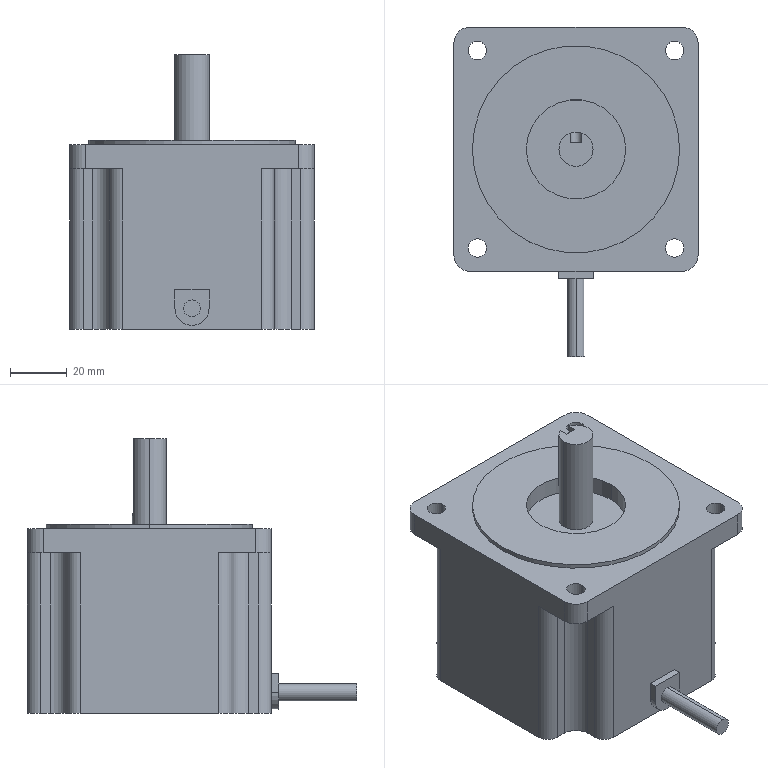Part | STEP file | JHSTM86-1.8-S-65-3 stepper motor MISUMI 657 | 1 solid | 66 faces | box 86 x 116 x 96.85 mm | volume 438131 mm3 | cylinder 36 | plane 30 | commonest cylinder face diameters 6.5 x8 9.2 x8 11 x4 11.8 x4 12 x3 6 x2